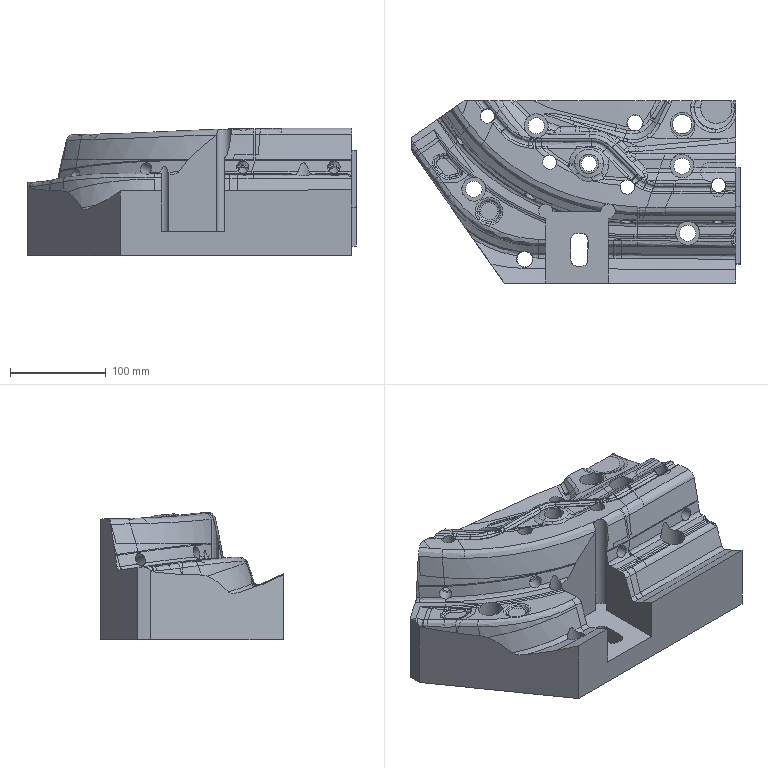Part | NX | features solid 2 | 1 solid | 448 faces | box 343.003 x 191.593 x 132.684 mm | volume 4957734 mm3 | spline 377 | plane 39 | cylinder 32 | commonest cylinder face diameters 15 x6 17 x6 25 x5 10 x4 13 x4 16 x3